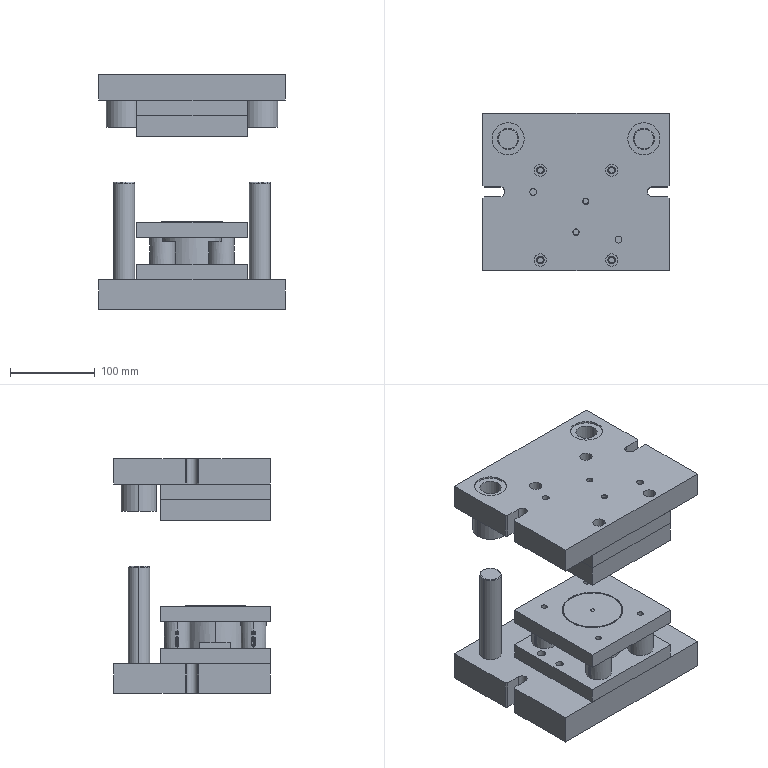Part | SolidWorks | 27 solids | 699 faces | box 220 x 185 x 276.914 mm | volume 4159283 mm3 | cylinder 344 | plane 187 | spline 100 | cone 54 | torus 14 | commonest cylinder face diameters 30 x136 6.806 x20 9.007 x20 14.5 x20 8 x14 25 x12